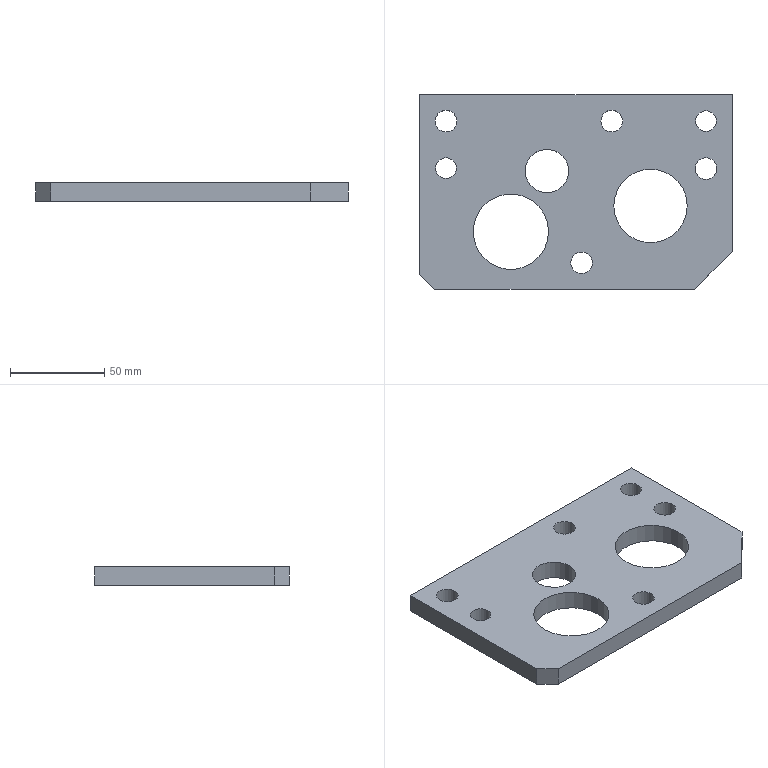Part | STEP file | lll_id4262_x_t | 1 solid | 17 faces | box 166 x 103.25 x 10 mm | volume 134346 mm3 | cylinder 9 | plane 8 | commonest cylinder face diameters 11.509 x4 11 x2 23 x1 39 x1 40 x1
STEP:
#1=CARTESIAN_POINT('',(3400.,57.,-45.));
#2=VERTEX_POINT('',#1);
#3=CARTESIAN_POINT('',(3419.5,57.,-45.));
#4=DIRECTION('',(0.,0.,1.));
#5=DIRECTION('',(-1.,0.,0.));
#6=AXIS2_PLACEMENT_3D('',#3,#4,#5);
#7=CIRCLE('',#6,19.5);
#8=EDGE_CURVE('',#2,#2,#7,.T.);
#9=ORIENTED_EDGE('',*,*,#8,.T.);
#10=EDGE_LOOP('',(#9));
#11=FACE_BOUND('',#10,.T.);
#12=CARTESIAN_POINT('',(3462.935,32.75,-45.));
#13=VERTEX_POINT('',#12);
#14=CARTESIAN_POINT('',(3462.935,116.,-45.));
#15=VERTEX_POINT('',#14);
#16=CARTESIAN_POINT('',(3462.935,215.25,-45.));
#17=DIRECTION('',(0.,1.,0.));
#18=VECTOR('',#17,1.);
#19=LINE('',#16,#18);
#20=EDGE_CURVE('',#13,#15,#19,.T.);
#21=ORIENTED_EDGE('',*,*,#20,.F.);
#22=CARTESIAN_POINT('',(3442.935,12.75,-45.));
#23=VERTEX_POINT('',#22);
#24=CARTESIAN_POINT('',(3455.935,25.75,-45.));
#25=DIRECTION('',(-0.7071,-0.7071,0.));
#26=VECTOR('',#25,1.);
#27=LINE('',#24,#26);
#28=EDGE_CURVE('',#13,#23,#27,.T.);
#29=ORIENTED_EDGE('',*,*,#28,.T.);
#30=CARTESIAN_POINT('',(3304.935,12.75,-45.));
#31=VERTEX_POINT('',#30);
#32=CARTESIAN_POINT('',(3266.435,12.75,-45.));
#33=DIRECTION('',(1.,0.,0.));
#34=VECTOR('',#33,1.);
#35=LINE('',#32,#34);
#36=EDGE_CURVE('',#31,#23,#35,.T.);
#37=ORIENTED_EDGE('',*,*,#36,.F.);
#38=CARTESIAN_POINT('',(3296.935,20.75,-45.));
#39=VERTEX_POINT('',#38);
#40=CARTESIAN_POINT('',(3179.435,138.25,-45.));
#41=DIRECTION('',(-0.7071,0.7071,0.));
#42=VECTOR('',#41,1.);
#43=LINE('',#40,#42);
#44=EDGE_CURVE('',#31,#39,#43,.T.);
#45=ORIENTED_EDGE('',*,*,#44,.T.);
#46=CARTESIAN_POINT('',(3296.935,116.,-45.));
#47=VERTEX_POINT('',#46);
#48=CARTESIAN_POINT('',(3296.935,215.25,-45.));
#49=DIRECTION('',(0.,-1.,0.));
#50=VECTOR('',#49,1.);
#51=LINE('',#48,#50);
#52=EDGE_CURVE('',#47,#39,#51,.T.);
#53=ORIENTED_EDGE('',*,*,#52,.F.);
#54=CARTESIAN_POINT('',(3266.435,116.,-45.));
#55=DIRECTION('',(-1.,0.,0.));
#56=VECTOR('',#55,1.);
#57=LINE('',#54,#56);
#58=EDGE_CURVE('',#15,#47,#57,.T.);
#59=ORIENTED_EDGE('',*,*,#58,.F.);
#60=EDGE_LOOP('',(#21,#29,#37,#45,#53,#59));
#61=FACE_BOUND('',#60,.T.);
#62=CARTESIAN_POINT('',(3305.181,102.,-45.));
#63=VERTEX_POINT('',#62);
#64=CARTESIAN_POINT('',(3310.935,102.,-45.));
#65=DIRECTION('',(0.,0.,-1.));
#66=DIRECTION('',(-1.,0.,0.));
#67=AXIS2_PLACEMENT_3D('',#64,#65,#66);
#68=CIRCLE('',#67,5.755);
#69=EDGE_CURVE('',#63,#63,#68,.T.);
#70=ORIENTED_EDGE('',*,*,#69,.F.);
#71=EDGE_LOOP('',(#70));
#72=FACE_BOUND('',#71,.T.);
#73=CARTESIAN_POINT('',(3305.435,77.,-45.));
#74=VERTEX_POINT('',#73);
#75=CARTESIAN_POINT('',(3310.935,77.,-45.));
#76=DIRECTION('',(0.,0.,-1.));
#77=DIRECTION('',(-1.,0.,0.));
#78=AXIS2_PLACEMENT_3D('',#75,#76,#77);
#79=CIRCLE('',#78,5.5);
#80=EDGE_CURVE('',#74,#74,#79,.T.);
#81=ORIENTED_EDGE('',*,*,#80,.F.);
#82=EDGE_LOOP('',(#81));
#83=FACE_BOUND('',#82,.T.);
#84=CARTESIAN_POINT('',(3377.181,26.75,-45.));
#85=VERTEX_POINT('',#84);
#86=CARTESIAN_POINT('',(3382.935,26.75,-45.));
#87=DIRECTION('',(0.,0.,-1.));
#88=DIRECTION('',(-1.,0.,0.));
#89=AXIS2_PLACEMENT_3D('',#86,#87,#88);
#90=CIRCLE('',#89,5.755);
#91=EDGE_CURVE('',#85,#85,#90,.T.);
#92=ORIENTED_EDGE('',*,*,#91,.F.);
#93=EDGE_LOOP('',(#92));
#94=FACE_BOUND('',#93,.T.);
#95=CARTESIAN_POINT('',(3443.435,102.,-45.));
#96=VERTEX_POINT('',#95);
#97=CARTESIAN_POINT('',(3448.935,102.,-45.));
#98=DIRECTION('',(0.,0.,-1.));
#99=DIRECTION('',(-1.,0.,0.));
#100=AXIS2_PLACEMENT_3D('',#97,#98,#99);
#101=CIRCLE('',#100,5.5);
#102=EDGE_CURVE('',#96,#96,#101,.T.);
#103=ORIENTED_EDGE('',*,*,#102,.F.);
#104=EDGE_LOOP('',(#103));
#105=FACE_BOUND('',#104,.T.);
#106=CARTESIAN_POINT('',(3393.181,102.,-45.));
#107=VERTEX_POINT('',#106);
#108=CARTESIAN_POINT('',(3398.935,102.,-45.));
#109=DIRECTION('',(0.,0.,-1.));
#110=DIRECTION('',(-1.,0.,0.));
#111=AXIS2_PLACEMENT_3D('',#108,#109,#110);
#112=CIRCLE('',#111,5.755);
#113=EDGE_CURVE('',#107,#107,#112,.T.);
#114=ORIENTED_EDGE('',*,*,#113,.F.);
#115=EDGE_LOOP('',(#114));
#116=FACE_BOUND('',#115,.T.);
#117=CARTESIAN_POINT('',(3443.181,76.75,-45.));
#118=VERTEX_POINT('',#117);
#119=CARTESIAN_POINT('',(3448.935,76.75,-45.));
#120=DIRECTION('',(0.,0.,-1.));
#121=DIRECTION('',(-1.,0.,0.));
#122=AXIS2_PLACEMENT_3D('',#119,#120,#121);
#123=CIRCLE('',#122,5.755);
#124=EDGE_CURVE('',#118,#118,#123,.T.);
#125=ORIENTED_EDGE('',*,*,#124,.F.);
#126=EDGE_LOOP('',(#125));
#127=FACE_BOUND('',#126,.T.);
#128=CARTESIAN_POINT('',(3353.,75.5,-45.));
#129=VERTEX_POINT('',#128);
#130=CARTESIAN_POINT('',(3364.5,75.5,-45.));
#131=DIRECTION('',(0.,0.,-1.));
#132=DIRECTION('',(-1.,0.,0.));
#133=AXIS2_PLACEMENT_3D('',#130,#131,#132);
#134=CIRCLE('',#133,11.5);
#135=EDGE_CURVE('',#129,#129,#134,.T.);
#136=ORIENTED_EDGE('',*,*,#135,.F.);
#137=EDGE_LOOP('',(#136));
#138=FACE_BOUND('',#137,.T.);
#139=CARTESIAN_POINT('',(3325.367,43.288,-45.));
#140=VERTEX_POINT('',#139);
#141=CARTESIAN_POINT('',(3345.367,43.288,-45.));
#142=DIRECTION('',(0.,0.,1.));
#143=DIRECTION('',(-1.,0.,0.));
#144=AXIS2_PLACEMENT_3D('',#141,#142,#143);
#145=CIRCLE('',#144,20.);
#146=EDGE_CURVE('',#140,#140,#145,.T.);
#147=ORIENTED_EDGE('',*,*,#146,.T.);
#148=EDGE_LOOP('',(#147));
#149=FACE_BOUND('',#148,.T.);
#150=CARTESIAN_POINT('',(3266.435,215.25,-45.));
#151=DIRECTION('',(0.,0.,-1.));
#152=DIRECTION('',(1.,0.,0.));
#153=AXIS2_PLACEMENT_3D('',#150,#151,#152);
#154=PLANE('',#153);
#155=ADVANCED_FACE('',(#11,#61,#72,#83,#94,#105,#116,#127,#138,#149),#154,.T.);
#156=CARTESIAN_POINT('',(3400.,57.,-35.));
#157=VERTEX_POINT('',#156);
#158=CARTESIAN_POINT('',(3419.5,57.,-35.));
#159=DIRECTION('',(0.,0.,1.));
#160=DIRECTION('',(-1.,0.,0.));
#161=AXIS2_PLACEMENT_3D('',#158,#159,#160);
#162=CIRCLE('',#161,19.5);
#163=EDGE_CURVE('',#157,#157,#162,.T.);
#164=ORIENTED_EDGE('',*,*,#163,.F.);
#165=EDGE_LOOP('',(#164));
#166=FACE_BOUND('',#165,.T.);
#167=CARTESIAN_POINT('',(3462.935,32.75,-35.));
#168=VERTEX_POINT('',#167);
#169=CARTESIAN_POINT('',(3462.935,116.,-35.));
#170=VERTEX_POINT('',#169);
#171=CARTESIAN_POINT('',(3462.935,215.25,-35.));
#172=DIRECTION('',(0.,1.,0.));
#173=VECTOR('',#172,1.);
#174=LINE('',#171,#173);
#175=EDGE_CURVE('',#168,#170,#174,.T.);
#176=ORIENTED_EDGE('',*,*,#175,.T.);
#177=CARTESIAN_POINT('',(3296.935,116.,-35.));
#178=VERTEX_POINT('',#177);
#179=CARTESIAN_POINT('',(3266.435,116.,-35.));
#180=DIRECTION('',(-1.,0.,0.));
#181=VECTOR('',#180,1.);
#182=LINE('',#179,#181);
#183=EDGE_CURVE('',#170,#178,#182,.T.);
#184=ORIENTED_EDGE('',*,*,#183,.T.);
#185=CARTESIAN_POINT('',(3296.935,20.75,-35.));
#186=VERTEX_POINT('',#185);
#187=CARTESIAN_POINT('',(3296.935,215.25,-35.));
#188=DIRECTION('',(0.,-1.,0.));
#189=VECTOR('',#188,1.);
#190=LINE('',#187,#189);
#191=EDGE_CURVE('',#178,#186,#190,.T.);
#192=ORIENTED_EDGE('',*,*,#191,.T.);
#193=CARTESIAN_POINT('',(3304.935,12.75,-35.));
#194=VERTEX_POINT('',#193);
#195=CARTESIAN_POINT('',(3179.435,138.25,-35.));
#196=DIRECTION('',(-0.7071,0.7071,0.));
#197=VECTOR('',#196,1.);
#198=LINE('',#195,#197);
#199=EDGE_CURVE('',#194,#186,#198,.T.);
#200=ORIENTED_EDGE('',*,*,#199,.F.);
#201=CARTESIAN_POINT('',(3442.935,12.75,-35.));
#202=VERTEX_POINT('',#201);
#203=CARTESIAN_POINT('',(3266.435,12.75,-35.));
#204=DIRECTION('',(1.,0.,0.));
#205=VECTOR('',#204,1.);
#206=LINE('',#203,#205);
#207=EDGE_CURVE('',#194,#202,#206,.T.);
#208=ORIENTED_EDGE('',*,*,#207,.T.);
#209=CARTESIAN_POINT('',(3455.935,25.75,-35.));
#210=DIRECTION('',(-0.7071,-0.7071,0.));
#211=VECTOR('',#210,1.);
#212=LINE('',#209,#211);
#213=EDGE_CURVE('',#168,#202,#212,.T.);
#214=ORIENTED_EDGE('',*,*,#213,.F.);
#215=EDGE_LOOP('',(#176,#184,#192,#200,#208,#214));
#216=FACE_BOUND('',#215,.T.);
#217=CARTESIAN_POINT('',(3305.181,102.,-35.));
#218=VERTEX_POINT('',#217);
#219=CARTESIAN_POINT('',(3310.935,102.,-35.));
#220=DIRECTION('',(0.,0.,-1.));
#221=DIRECTION('',(-1.,0.,0.));
#222=AXIS2_PLACEMENT_3D('',#219,#220,#221);
#223=CIRCLE('',#222,5.755);
#224=EDGE_CURVE('',#218,#218,#223,.T.);
#225=ORIENTED_EDGE('',*,*,#224,.T.);
#226=EDGE_LOOP('',(#225));
#227=FACE_BOUND('',#226,.T.);
#228=CARTESIAN_POINT('',(3305.435,77.,-35.));
#229=VERTEX_POINT('',#228);
#230=CARTESIAN_POINT('',(3310.935,77.,-35.));
#231=DIRECTION('',(0.,0.,-1.));
#232=DIRECTION('',(-1.,0.,0.));
#233=AXIS2_PLACEMENT_3D('',#230,#231,#232);
#234=CIRCLE('',#233,5.5);
#235=EDGE_CURVE('',#229,#229,#234,.T.);
#236=ORIENTED_EDGE('',*,*,#235,.T.);
#237=EDGE_LOOP('',(#236));
#238=FACE_BOUND('',#237,.T.);
#239=CARTESIAN_POINT('',(3377.181,26.75,-35.));
#240=VERTEX_POINT('',#239);
#241=CARTESIAN_POINT('',(3382.935,26.75,-35.));
#242=DIRECTION('',(0.,0.,-1.));
#243=DIRECTION('',(-1.,0.,0.));
#244=AXIS2_PLACEMENT_3D('',#241,#242,#243);
#245=CIRCLE('',#244,5.755);
#246=EDGE_CURVE('',#240,#240,#245,.T.);
#247=ORIENTED_EDGE('',*,*,#246,.T.);
#248=EDGE_LOOP('',(#247));
#249=FACE_BOUND('',#248,.T.);
#250=CARTESIAN_POINT('',(3443.435,102.,-35.));
#251=VERTEX_POINT('',#250);
#252=CARTESIAN_POINT('',(3448.935,102.,-35.));
#253=DIRECTION('',(0.,0.,-1.));
#254=DIRECTION('',(-1.,0.,0.));
#255=AXIS2_PLACEMENT_3D('',#252,#253,#254);
#256=CIRCLE('',#255,5.5);
#257=EDGE_CURVE('',#251,#251,#256,.T.);
#258=ORIENTED_EDGE('',*,*,#257,.T.);
#259=EDGE_LOOP('',(#258));
#260=FACE_BOUND('',#259,.T.);
#261=CARTESIAN_POINT('',(3393.181,102.,-35.));
#262=VERTEX_POINT('',#261);
#263=CARTESIAN_POINT('',(3398.935,102.,-35.));
#264=DIRECTION('',(0.,0.,-1.));
#265=DIRECTION('',(-1.,0.,0.));
#266=AXIS2_PLACEMENT_3D('',#263,#264,#265);
#267=CIRCLE('',#266,5.755);
#268=EDGE_CURVE('',#262,#262,#267,.T.);
#269=ORIENTED_EDGE('',*,*,#268,.T.);
#270=EDGE_LOOP('',(#269));
#271=FACE_BOUND('',#270,.T.);
#272=CARTESIAN_POINT('',(3443.181,76.75,-35.));
#273=VERTEX_POINT('',#272);
#274=CARTESIAN_POINT('',(3448.935,76.75,-35.));
#275=DIRECTION('',(0.,0.,-1.));
#276=DIRECTION('',(-1.,0.,0.));
#277=AXIS2_PLACEMENT_3D('',#274,#275,#276);
#278=CIRCLE('',#277,5.755);
#279=EDGE_CURVE('',#273,#273,#278,.T.);
#280=ORIENTED_EDGE('',*,*,#279,.T.);
#281=EDGE_LOOP('',(#280));
#282=FACE_BOUND('',#281,.T.);
#283=CARTESIAN_POINT('',(3353.,75.5,-35.));
#284=VERTEX_POINT('',#283);
#285=CARTESIAN_POINT('',(3364.5,75.5,-35.));
#286=DIRECTION('',(0.,0.,-1.));
#287=DIRECTION('',(-1.,0.,0.));
#288=AXIS2_PLACEMENT_3D('',#285,#286,#287);
#289=CIRCLE('',#288,11.5);
#290=EDGE_CURVE('',#284,#284,#289,.T.);
#291=ORIENTED_EDGE('',*,*,#290,.T.);
#292=EDGE_LOOP('',(#291));
#293=FACE_BOUND('',#292,.T.);
#294=CARTESIAN_POINT('',(3325.367,43.288,-35.));
#295=VERTEX_POINT('',#294);
#296=CARTESIAN_POINT('',(3345.367,43.288,-35.));
#297=DIRECTION('',(0.,0.,1.));
#298=DIRECTION('',(-1.,0.,0.));
#299=AXIS2_PLACEMENT_3D('',#296,#297,#298);
#300=CIRCLE('',#299,20.);
#301=EDGE_CURVE('',#295,#295,#300,.T.);
#302=ORIENTED_EDGE('',*,*,#301,.F.);
#303=EDGE_LOOP('',(#302));
#304=FACE_BOUND('',#303,.T.);
#305=CARTESIAN_POINT('',(3266.435,215.25,-35.));
#306=DIRECTION('',(0.,0.,-1.));
#307=DIRECTION('',(1.,0.,0.));
#308=AXIS2_PLACEMENT_3D('',#305,#306,#307);
#309=PLANE('',#308);
#310=ADVANCED_FACE('',(#166,#216,#227,#238,#249,#260,#271,#282,#293,#304),#309,.F.);
#311=ORIENTED_EDGE('',*,*,#163,.T.);
#312=EDGE_LOOP('',(#311));
#313=FACE_BOUND('',#312,.T.);
#314=ORIENTED_EDGE('',*,*,#8,.F.);
#315=EDGE_LOOP('',(#314));
#316=FACE_BOUND('',#315,.T.);
#317=CARTESIAN_POINT('',(3419.5,57.,-35.));
#318=DIRECTION('',(0.,0.,-1.));
#319=DIRECTION('',(-1.,0.,0.));
#320=AXIS2_PLACEMENT_3D('',#317,#318,#319);
#321=CYLINDRICAL_SURFACE('',#320,19.5);
#322=ADVANCED_FACE('',(#313,#316),#321,.F.);
#323=CARTESIAN_POINT('',(3442.935,12.75,-35.));
#324=DIRECTION('',(0.,0.,-1.));
#325=VECTOR('',#324,1.);
#326=LINE('',#323,#325);
#327=EDGE_CURVE('',#202,#23,#326,.T.);
#328=ORIENTED_EDGE('',*,*,#327,.F.);
#329=ORIENTED_EDGE('',*,*,#207,.F.);
#330=CARTESIAN_POINT('',(3304.935,12.75,-35.));
#331=DIRECTION('',(0.,0.,-1.));
#332=VECTOR('',#331,1.);
#333=LINE('',#330,#332);
#334=EDGE_CURVE('',#194,#31,#333,.T.);
#335=ORIENTED_EDGE('',*,*,#334,.T.);
#336=ORIENTED_EDGE('',*,*,#36,.T.);
#337=EDGE_LOOP('',(#328,#329,#335,#336));
#338=FACE_OUTER_BOUND('',#337,.T.);
#339=CARTESIAN_POINT('',(3266.435,12.75,-35.));
#340=DIRECTION('',(0.,1.,0.));
#341=DIRECTION('',(1.,0.,0.));
#342=AXIS2_PLACEMENT_3D('',#339,#340,#341);
#343=PLANE('',#342);
#344=ADVANCED_FACE('',(#338),#343,.F.);
#345=ORIENTED_EDGE('',*,*,#334,.F.);
#346=ORIENTED_EDGE('',*,*,#199,.T.);
#347=CARTESIAN_POINT('',(3296.935,20.75,-35.));
#348=DIRECTION('',(0.,0.,-1.));
#349=VECTOR('',#348,1.);
#350=LINE('',#347,#349);
#351=EDGE_CURVE('',#186,#39,#350,.T.);
#352=ORIENTED_EDGE('',*,*,#351,.T.);
#353=ORIENTED_EDGE('',*,*,#44,.F.);
#354=EDGE_LOOP('',(#345,#346,#352,#353));
#355=FACE_OUTER_BOUND('',#354,.T.);
#356=CARTESIAN_POINT('',(3179.435,138.25,-35.));
#357=DIRECTION('',(-0.7071,-0.7071,0.));
#358=DIRECTION('',(-0.7071,0.7071,0.));
#359=AXIS2_PLACEMENT_3D('',#356,#357,#358);
#360=PLANE('',#359);
#361=ADVANCED_FACE('',(#355),#360,.T.);
#362=ORIENTED_EDGE('',*,*,#351,.F.);
#363=ORIENTED_EDGE('',*,*,#191,.F.);
#364=CARTESIAN_POINT('',(3296.935,116.,-35.));
#365=DIRECTION('',(0.,0.,-1.));
#366=VECTOR('',#365,1.);
#367=LINE('',#364,#366);
#368=EDGE_CURVE('',#178,#47,#367,.T.);
#369=ORIENTED_EDGE('',*,*,#368,.T.);
#370=ORIENTED_EDGE('',*,*,#52,.T.);
#371=EDGE_LOOP('',(#362,#363,#369,#370));
#372=FACE_OUTER_BOUND('',#371,.T.);
#373=CARTESIAN_POINT('',(3296.935,215.25,-35.));
#374=DIRECTION('',(1.,0.,0.));
#375=DIRECTION('',(0.,-1.,0.));
#376=AXIS2_PLACEMENT_3D('',#373,#374,#375);
#377=PLANE('',#376);
#378=ADVANCED_FACE('',(#372),#377,.F.);
#379=ORIENTED_EDGE('',*,*,#368,.F.);
#380=ORIENTED_EDGE('',*,*,#183,.F.);
#381=CARTESIAN_POINT('',(3462.935,116.,-35.));
#382=DIRECTION('',(0.,0.,-1.));
#383=VECTOR('',#382,1.);
#384=LINE('',#381,#383);
#385=EDGE_CURVE('',#170,#15,#384,.T.);
#386=ORIENTED_EDGE('',*,*,#385,.T.);
#387=ORIENTED_EDGE('',*,*,#58,.T.);
#388=EDGE_LOOP('',(#379,#380,#386,#387));
#389=FACE_OUTER_BOUND('',#388,.T.);
#390=CARTESIAN_POINT('',(3266.435,116.,-35.));
#391=DIRECTION('',(0.,-1.,0.));
#392=DIRECTION('',(-1.,0.,0.));
#393=AXIS2_PLACEMENT_3D('',#390,#391,#392);
#394=PLANE('',#393);
#395=ADVANCED_FACE('',(#389),#394,.F.);
#396=ORIENTED_EDGE('',*,*,#385,.F.);
#397=ORIENTED_EDGE('',*,*,#175,.F.);
#398=CARTESIAN_POINT('',(3462.935,32.75,-35.));
#399=DIRECTION('',(0.,0.,-1.));
#400=VECTOR('',#399,1.);
#401=LINE('',#398,#400);
#402=EDGE_CURVE('',#168,#13,#401,.T.);
#403=ORIENTED_EDGE('',*,*,#402,.T.);
#404=ORIENTED_EDGE('',*,*,#20,.T.);
#405=EDGE_LOOP('',(#396,#397,#403,#404));
#406=FACE_OUTER_BOUND('',#405,.T.);
#407=CARTESIAN_POINT('',(3462.935,215.25,-35.));
#408=DIRECTION('',(-1.,0.,0.));
#409=DIRECTION('',(0.,1.,0.));
#410=AXIS2_PLACEMENT_3D('',#407,#408,#409);
#411=PLANE('',#410);
#412=ADVANCED_FACE('',(#406),#411,.F.);
#413=ORIENTED_EDGE('',*,*,#124,.T.);
#414=EDGE_LOOP('',(#413));
#415=FACE_BOUND('',#414,.T.);
#416=ORIENTED_EDGE('',*,*,#279,.F.);
#417=EDGE_LOOP('',(#416));
#418=FACE_BOUND('',#417,.T.);
#419=CARTESIAN_POINT('',(3448.935,76.75,-35.));
#420=DIRECTION('',(0.,0.,-1.));
#421=DIRECTION('',(-1.,0.,0.));
#422=AXIS2_PLACEMENT_3D('',#419,#420,#421);
#423=CYLINDRICAL_SURFACE('',#422,5.755);
#424=ADVANCED_FACE('',(#415,#418),#423,.F.);
#425=ORIENTED_EDGE('',*,*,#113,.T.);
#426=EDGE_LOOP('',(#425));
#427=FACE_BOUND('',#426,.T.);
#428=ORIENTED_EDGE('',*,*,#268,.F.);
#429=EDGE_LOOP('',(#428));
#430=FACE_BOUND('',#429,.T.);
#431=CARTESIAN_POINT('',(3398.935,102.,-35.));
#432=DIRECTION('',(0.,0.,-1.));
#433=DIRECTION('',(-1.,0.,0.));
#434=AXIS2_PLACEMENT_3D('',#431,#432,#433);
#435=CYLINDRICAL_SURFACE('',#434,5.755);
#436=ADVANCED_FACE('',(#427,#430),#435,.F.);
#437=ORIENTED_EDGE('',*,*,#102,.T.);
#438=EDGE_LOOP('',(#437));
#439=FACE_BOUND('',#438,.T.);
#440=ORIENTED_EDGE('',*,*,#257,.F.);
#441=EDGE_LOOP('',(#440));
#442=FACE_BOUND('',#441,.T.);
#443=CARTESIAN_POINT('',(3448.935,102.,-35.));
#444=DIRECTION('',(0.,0.,-1.));
#445=DIRECTION('',(-1.,0.,0.));
#446=AXIS2_PLACEMENT_3D('',#443,#444,#445);
#447=CYLINDRICAL_SURFACE('',#446,5.5);
#448=ADVANCED_FACE('',(#439,#442),#447,.F.);
#449=ORIENTED_EDGE('',*,*,#91,.T.);
#450=EDGE_LOOP('',(#449));
#451=FACE_BOUND('',#450,.T.);
#452=ORIENTED_EDGE('',*,*,#246,.F.);
#453=EDGE_LOOP('',(#452));
#454=FACE_BOUND('',#453,.T.);
#455=CARTESIAN_POINT('',(3382.935,26.75,-35.));
#456=DIRECTION('',(0.,0.,-1.));
#457=DIRECTION('',(-1.,0.,0.));
#458=AXIS2_PLACEMENT_3D('',#455,#456,#457);
#459=CYLINDRICAL_SURFACE('',#458,5.755);
#460=ADVANCED_FACE('',(#451,#454),#459,.F.);
#461=ORIENTED_EDGE('',*,*,#80,.T.);
#462=EDGE_LOOP('',(#461));
#463=FACE_BOUND('',#462,.T.);
#464=ORIENTED_EDGE('',*,*,#235,.F.);
#465=EDGE_LOOP('',(#464));
#466=FACE_BOUND('',#465,.T.);
#467=CARTESIAN_POINT('',(3310.935,77.,-35.));
#468=DIRECTION('',(0.,0.,-1.));
#469=DIRECTION('',(-1.,0.,0.));
#470=AXIS2_PLACEMENT_3D('',#467,#468,#469);
#471=CYLINDRICAL_SURFACE('',#470,5.5);
#472=ADVANCED_FACE('',(#463,#466),#471,.F.);
#473=ORIENTED_EDGE('',*,*,#69,.T.);
#474=EDGE_LOOP('',(#473));
#475=FACE_BOUND('',#474,.T.);
#476=ORIENTED_EDGE('',*,*,#224,.F.);
#477=EDGE_LOOP('',(#476));
#478=FACE_BOUND('',#477,.T.);
#479=CARTESIAN_POINT('',(3310.935,102.,-35.));
#480=DIRECTION('',(0.,0.,-1.));
#481=DIRECTION('',(-1.,0.,0.));
#482=AXIS2_PLACEMENT_3D('',#479,#480,#481);
#483=CYLINDRICAL_SURFACE('',#482,5.755);
#484=ADVANCED_FACE('',(#475,#478),#483,.F.);
#485=ORIENTED_EDGE('',*,*,#213,.T.);
#486=ORIENTED_EDGE('',*,*,#327,.T.);
#487=ORIENTED_EDGE('',*,*,#28,.F.);
#488=ORIENTED_EDGE('',*,*,#402,.F.);
#489=EDGE_LOOP('',(#485,#486,#487,#488));
#490=FACE_OUTER_BOUND('',#489,.T.);
#491=CARTESIAN_POINT('',(3455.935,25.75,-35.));
#492=DIRECTION('',(-0.7071,0.7071,0.));
#493=DIRECTION('',(0.7071,0.7071,0.));
#494=AXIS2_PLACEMENT_3D('',#491,#492,#493);
#495=PLANE('',#494);
#496=ADVANCED_FACE('',(#490),#495,.F.);
#497=ORIENTED_EDGE('',*,*,#135,.T.);
#498=EDGE_LOOP('',(#497));
#499=FACE_BOUND('',#498,.T.);
#500=ORIENTED_EDGE('',*,*,#290,.F.);
#501=EDGE_LOOP('',(#500));
#502=FACE_BOUND('',#501,.T.);
#503=CARTESIAN_POINT('',(3364.5,75.5,-235.));
#504=DIRECTION('',(0.,0.,1.));
#505=DIRECTION('',(1.,0.,0.));
#506=AXIS2_PLACEMENT_3D('',#503,#504,#505);
#507=CYLINDRICAL_SURFACE('',#506,11.5);
#508=ADVANCED_FACE('',(#499,#502),#507,.F.);
#509=ORIENTED_EDGE('',*,*,#146,.F.);
#510=EDGE_LOOP('',(#509));
#511=FACE_BOUND('',#510,.T.);
#512=ORIENTED_EDGE('',*,*,#301,.T.);
#513=EDGE_LOOP('',(#512));
#514=FACE_BOUND('',#513,.T.);
#515=CARTESIAN_POINT('',(3345.367,43.288,-235.));
#516=DIRECTION('',(0.,0.,1.));
#517=DIRECTION('',(1.,0.,0.));
#518=AXIS2_PLACEMENT_3D('',#515,#516,#517);
#519=CYLINDRICAL_SURFACE('',#518,20.);
#520=ADVANCED_FACE('',(#511,#514),#519,.F.);
#521=CLOSED_SHELL('',(#155,#310,#322,#344,#361,#378,#395,#412,#424,#436,#448,#460,#472,#484,#496,#508,#520));
#522=MANIFOLD_SOLID_BREP('',#521);
#523=(LENGTH_UNIT()NAMED_UNIT(*)SI_UNIT(.MILLI.,.METRE.));
#524=UNCERTAINTY_MEASURE_WITH_UNIT(LENGTH_MEASURE(0.00002),#523,'','');
#525=(NAMED_UNIT(*)PLANE_ANGLE_UNIT()SI_UNIT($,.RADIAN.));
#526=PLANE_ANGLE_MEASURE_WITH_UNIT(PLANE_ANGLE_MEASURE(0.01745),#525);
#527=DIMENSIONAL_EXPONENTS(0.,0.,0.,0.,0.,0.,0.);
#528=(CONVERSION_BASED_UNIT('DEGREE',#526)NAMED_UNIT(#527)PLANE_ANGLE_UNIT());
#529=(NAMED_UNIT(*)SI_UNIT($,.STERADIAN.)SOLID_ANGLE_UNIT());
#530=(GEOMETRIC_REPRESENTATION_CONTEXT(3)GLOBAL_UNCERTAINTY_ASSIGNED_CONTEXT((#524))GLOBAL_UNIT_ASSIGNED_CONTEXT((#523,#528,#529))REPRESENTATION_CONTEXT('',''));
#531=ADVANCED_BREP_SHAPE_REPRESENTATION('',(#522),#530);